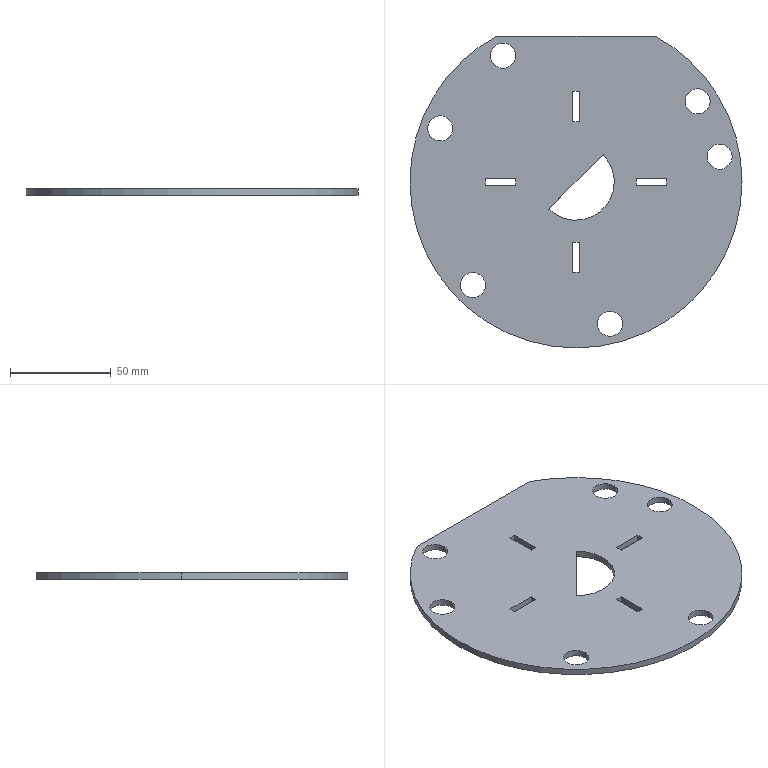Part | SolidWorks | features FlatPattern 1, SMBaseFlange 1, SheetMetal 1 | 1 solid | 36 faces | box 165 x 155 x 3.2 mm | volume 61928 mm3 | plane 20 | cylinder 16 | commonest cylinder face diameters 12.5 x12 165 x3 38.1 x1
STEP:
#1=CARTESIAN_POINT('',(2.418,-3.235,3.2));
#2=VERTEX_POINT('',#1);
#3=CARTESIAN_POINT('',(14.918,-3.235,3.2));
#4=VERTEX_POINT('',#3);
#5=CARTESIAN_POINT('',(8.668,-3.235,3.2));
#6=DIRECTION('',(0.,0.,1.));
#7=DIRECTION('',(1.,0.,0.));
#8=AXIS2_PLACEMENT_3D('',#5,#6,#7);
#9=CIRCLE('',#8,6.25);
#10=EDGE_CURVE('',#2,#4,#9,.T.);
#11=ORIENTED_EDGE('',*,*,#10,.T.);
#12=CARTESIAN_POINT('',(14.918,-3.235,0.));
#13=VERTEX_POINT('',#12);
#14=CARTESIAN_POINT('',(14.918,-3.235,3.2));
#15=DIRECTION('',(0.,0.,-1.));
#16=VECTOR('',#15,1000.);
#17=LINE('',#14,#16);
#18=EDGE_CURVE('',#4,#13,#17,.T.);
#19=ORIENTED_EDGE('',*,*,#18,.T.);
#20=CARTESIAN_POINT('',(2.418,-3.235,0.));
#21=VERTEX_POINT('',#20);
#22=CARTESIAN_POINT('',(8.668,-3.235,0.));
#23=DIRECTION('',(0.,0.,1.));
#24=DIRECTION('',(1.,0.,0.));
#25=AXIS2_PLACEMENT_3D('',#22,#23,#24);
#26=CIRCLE('',#25,6.25);
#27=EDGE_CURVE('',#21,#13,#26,.T.);
#28=ORIENTED_EDGE('',*,*,#27,.F.);
#29=CARTESIAN_POINT('',(2.418,-3.235,3.2));
#30=DIRECTION('',(0.,0.,-1.));
#31=VECTOR('',#30,1000.);
#32=LINE('',#29,#31);
#33=EDGE_CURVE('',#2,#21,#32,.T.);
#34=ORIENTED_EDGE('',*,*,#33,.F.);
#35=EDGE_LOOP('',(#11,#19,#28,#34));
#36=FACE_OUTER_BOUND('',#35,.T.);
#37=CARTESIAN_POINT('',(8.668,-3.235,3.2));
#38=DIRECTION('',(0.,0.,-1.));
#39=DIRECTION('',(-1.,0.,0.));
#40=AXIS2_PLACEMENT_3D('',#37,#38,#39);
#41=CYLINDRICAL_SURFACE('',#40,6.25);
#42=ADVANCED_FACE('',(#36),#41,.F.);
#43=CARTESIAN_POINT('',(-8.524,24.191,3.2));
#44=VERTEX_POINT('',#43);
#45=CARTESIAN_POINT('',(3.976,24.191,3.2));
#46=VERTEX_POINT('',#45);
#47=CARTESIAN_POINT('',(-2.274,24.191,3.2));
#48=DIRECTION('',(0.,0.,1.));
#49=DIRECTION('',(1.,0.,0.));
#50=AXIS2_PLACEMENT_3D('',#47,#48,#49);
#51=CIRCLE('',#50,6.25);
#52=EDGE_CURVE('',#44,#46,#51,.T.);
#53=ORIENTED_EDGE('',*,*,#52,.T.);
#54=CARTESIAN_POINT('',(3.976,24.191,0.));
#55=VERTEX_POINT('',#54);
#56=CARTESIAN_POINT('',(3.976,24.191,3.2));
#57=DIRECTION('',(0.,0.,-1.));
#58=VECTOR('',#57,1000.);
#59=LINE('',#56,#58);
#60=EDGE_CURVE('',#46,#55,#59,.T.);
#61=ORIENTED_EDGE('',*,*,#60,.T.);
#62=CARTESIAN_POINT('',(-8.524,24.191,0.));
#63=VERTEX_POINT('',#62);
#64=CARTESIAN_POINT('',(-2.274,24.191,0.));
#65=DIRECTION('',(0.,0.,1.));
#66=DIRECTION('',(1.,0.,0.));
#67=AXIS2_PLACEMENT_3D('',#64,#65,#66);
#68=CIRCLE('',#67,6.25);
#69=EDGE_CURVE('',#63,#55,#68,.T.);
#70=ORIENTED_EDGE('',*,*,#69,.F.);
#71=CARTESIAN_POINT('',(-8.524,24.191,3.2));
#72=DIRECTION('',(0.,0.,-1.));
#73=VECTOR('',#72,1000.);
#74=LINE('',#71,#73);
#75=EDGE_CURVE('',#44,#63,#74,.T.);
#76=ORIENTED_EDGE('',*,*,#75,.F.);
#77=EDGE_LOOP('',(#53,#61,#70,#76));
#78=FACE_OUTER_BOUND('',#77,.T.);
#79=CARTESIAN_POINT('',(-2.274,24.191,3.2));
#80=DIRECTION('',(0.,0.,-1.));
#81=DIRECTION('',(-1.,0.,0.));
#82=AXIS2_PLACEMENT_3D('',#79,#80,#81);
#83=CYLINDRICAL_SURFACE('',#82,6.25);
#84=ADVANCED_FACE('',(#78),#83,.F.);
#85=CARTESIAN_POINT('',(-105.231,46.962,3.2));
#86=VERTEX_POINT('',#85);
#87=CARTESIAN_POINT('',(-92.731,46.962,3.2));
#88=VERTEX_POINT('',#87);
#89=CARTESIAN_POINT('',(-98.981,46.962,3.2));
#90=DIRECTION('',(0.,0.,1.));
#91=DIRECTION('',(1.,0.,0.));
#92=AXIS2_PLACEMENT_3D('',#89,#90,#91);
#93=CIRCLE('',#92,6.25);
#94=EDGE_CURVE('',#86,#88,#93,.T.);
#95=ORIENTED_EDGE('',*,*,#94,.T.);
#96=CARTESIAN_POINT('',(-92.731,46.962,0.));
#97=VERTEX_POINT('',#96);
#98=CARTESIAN_POINT('',(-92.731,46.962,3.2));
#99=DIRECTION('',(0.,0.,-1.));
#100=VECTOR('',#99,1000.);
#101=LINE('',#98,#100);
#102=EDGE_CURVE('',#88,#97,#101,.T.);
#103=ORIENTED_EDGE('',*,*,#102,.T.);
#104=CARTESIAN_POINT('',(-105.231,46.962,0.));
#105=VERTEX_POINT('',#104);
#106=CARTESIAN_POINT('',(-98.981,46.962,0.));
#107=DIRECTION('',(0.,0.,1.));
#108=DIRECTION('',(1.,0.,0.));
#109=AXIS2_PLACEMENT_3D('',#106,#107,#108);
#110=CIRCLE('',#109,6.25);
#111=EDGE_CURVE('',#105,#97,#110,.T.);
#112=ORIENTED_EDGE('',*,*,#111,.F.);
#113=CARTESIAN_POINT('',(-105.231,46.962,3.2));
#114=DIRECTION('',(0.,0.,-1.));
#115=VECTOR('',#114,1000.);
#116=LINE('',#113,#115);
#117=EDGE_CURVE('',#86,#105,#116,.T.);
#118=ORIENTED_EDGE('',*,*,#117,.F.);
#119=EDGE_LOOP('',(#95,#103,#112,#118));
#120=FACE_OUTER_BOUND('',#119,.T.);
#121=CARTESIAN_POINT('',(-98.981,46.962,3.2));
#122=DIRECTION('',(0.,0.,-1.));
#123=DIRECTION('',(-1.,0.,0.));
#124=AXIS2_PLACEMENT_3D('',#121,#122,#123);
#125=CYLINDRICAL_SURFACE('',#124,6.25);
#126=ADVANCED_FACE('',(#120),#125,.F.);
#127=CARTESIAN_POINT('',(-136.436,10.747,3.2));
#128=VERTEX_POINT('',#127);
#129=CARTESIAN_POINT('',(-123.936,10.747,3.2));
#130=VERTEX_POINT('',#129);
#131=CARTESIAN_POINT('',(-130.186,10.747,3.2));
#132=DIRECTION('',(0.,0.,1.));
#133=DIRECTION('',(1.,0.,0.));
#134=AXIS2_PLACEMENT_3D('',#131,#132,#133);
#135=CIRCLE('',#134,6.25);
#136=EDGE_CURVE('',#128,#130,#135,.T.);
#137=ORIENTED_EDGE('',*,*,#136,.T.);
#138=CARTESIAN_POINT('',(-123.936,10.747,0.));
#139=VERTEX_POINT('',#138);
#140=CARTESIAN_POINT('',(-123.936,10.747,3.2));
#141=DIRECTION('',(0.,0.,-1.));
#142=VECTOR('',#141,1000.);
#143=LINE('',#140,#142);
#144=EDGE_CURVE('',#130,#139,#143,.T.);
#145=ORIENTED_EDGE('',*,*,#144,.T.);
#146=CARTESIAN_POINT('',(-136.436,10.747,0.));
#147=VERTEX_POINT('',#146);
#148=CARTESIAN_POINT('',(-130.186,10.747,0.));
#149=DIRECTION('',(0.,0.,1.));
#150=DIRECTION('',(1.,0.,0.));
#151=AXIS2_PLACEMENT_3D('',#148,#149,#150);
#152=CIRCLE('',#151,6.25);
#153=EDGE_CURVE('',#147,#139,#152,.T.);
#154=ORIENTED_EDGE('',*,*,#153,.F.);
#155=CARTESIAN_POINT('',(-136.436,10.747,3.2));
#156=DIRECTION('',(0.,0.,-1.));
#157=VECTOR('',#156,1000.);
#158=LINE('',#155,#157);
#159=EDGE_CURVE('',#128,#147,#158,.T.);
#160=ORIENTED_EDGE('',*,*,#159,.F.);
#161=EDGE_LOOP('',(#137,#145,#154,#160));
#162=FACE_OUTER_BOUND('',#161,.T.);
#163=CARTESIAN_POINT('',(-130.186,10.747,3.2));
#164=DIRECTION('',(0.,0.,-1.));
#165=DIRECTION('',(-1.,0.,0.));
#166=AXIS2_PLACEMENT_3D('',#163,#164,#165);
#167=CYLINDRICAL_SURFACE('',#166,6.25);
#168=ADVANCED_FACE('',(#162),#167,.F.);
#169=CARTESIAN_POINT('',(-120.246,-67.09,3.2));
#170=VERTEX_POINT('',#169);
#171=CARTESIAN_POINT('',(-107.746,-67.09,3.2));
#172=VERTEX_POINT('',#171);
#173=CARTESIAN_POINT('',(-113.996,-67.09,3.2));
#174=DIRECTION('',(0.,0.,1.));
#175=DIRECTION('',(1.,0.,0.));
#176=AXIS2_PLACEMENT_3D('',#173,#174,#175);
#177=CIRCLE('',#176,6.25);
#178=EDGE_CURVE('',#170,#172,#177,.T.);
#179=ORIENTED_EDGE('',*,*,#178,.T.);
#180=CARTESIAN_POINT('',(-107.746,-67.09,0.));
#181=VERTEX_POINT('',#180);
#182=CARTESIAN_POINT('',(-107.746,-67.09,3.2));
#183=DIRECTION('',(0.,0.,-1.));
#184=VECTOR('',#183,1000.);
#185=LINE('',#182,#184);
#186=EDGE_CURVE('',#172,#181,#185,.T.);
#187=ORIENTED_EDGE('',*,*,#186,.T.);
#188=CARTESIAN_POINT('',(-120.246,-67.09,0.));
#189=VERTEX_POINT('',#188);
#190=CARTESIAN_POINT('',(-113.996,-67.09,0.));
#191=DIRECTION('',(0.,0.,1.));
#192=DIRECTION('',(1.,0.,0.));
#193=AXIS2_PLACEMENT_3D('',#190,#191,#192);
#194=CIRCLE('',#193,6.25);
#195=EDGE_CURVE('',#189,#181,#194,.T.);
#196=ORIENTED_EDGE('',*,*,#195,.F.);
#197=CARTESIAN_POINT('',(-120.246,-67.09,3.2));
#198=DIRECTION('',(0.,0.,-1.));
#199=VECTOR('',#198,1000.);
#200=LINE('',#197,#199);
#201=EDGE_CURVE('',#170,#189,#200,.T.);
#202=ORIENTED_EDGE('',*,*,#201,.F.);
#203=EDGE_LOOP('',(#179,#187,#196,#202));
#204=FACE_OUTER_BOUND('',#203,.T.);
#205=CARTESIAN_POINT('',(-113.996,-67.09,3.2));
#206=DIRECTION('',(0.,0.,-1.));
#207=DIRECTION('',(-1.,0.,0.));
#208=AXIS2_PLACEMENT_3D('',#205,#206,#207);
#209=CYLINDRICAL_SURFACE('',#208,6.25);
#210=ADVANCED_FACE('',(#204),#209,.F.);
#211=CARTESIAN_POINT('',(-52.056,-86.321,3.2));
#212=VERTEX_POINT('',#211);
#213=CARTESIAN_POINT('',(-39.556,-86.321,3.2));
#214=VERTEX_POINT('',#213);
#215=CARTESIAN_POINT('',(-45.806,-86.321,3.2));
#216=DIRECTION('',(0.,0.,1.));
#217=DIRECTION('',(1.,0.,0.));
#218=AXIS2_PLACEMENT_3D('',#215,#216,#217);
#219=CIRCLE('',#218,6.25);
#220=EDGE_CURVE('',#212,#214,#219,.T.);
#221=ORIENTED_EDGE('',*,*,#220,.T.);
#222=CARTESIAN_POINT('',(-39.556,-86.321,0.));
#223=VERTEX_POINT('',#222);
#224=CARTESIAN_POINT('',(-39.556,-86.321,3.2));
#225=DIRECTION('',(0.,0.,-1.));
#226=VECTOR('',#225,1000.);
#227=LINE('',#224,#226);
#228=EDGE_CURVE('',#214,#223,#227,.T.);
#229=ORIENTED_EDGE('',*,*,#228,.T.);
#230=CARTESIAN_POINT('',(-52.056,-86.321,0.));
#231=VERTEX_POINT('',#230);
#232=CARTESIAN_POINT('',(-45.806,-86.321,0.));
#233=DIRECTION('',(0.,0.,1.));
#234=DIRECTION('',(1.,0.,0.));
#235=AXIS2_PLACEMENT_3D('',#232,#233,#234);
#236=CIRCLE('',#235,6.25);
#237=EDGE_CURVE('',#231,#223,#236,.T.);
#238=ORIENTED_EDGE('',*,*,#237,.F.);
#239=CARTESIAN_POINT('',(-52.056,-86.321,3.2));
#240=DIRECTION('',(0.,0.,-1.));
#241=VECTOR('',#240,1000.);
#242=LINE('',#239,#241);
#243=EDGE_CURVE('',#212,#231,#242,.T.);
#244=ORIENTED_EDGE('',*,*,#243,.F.);
#245=EDGE_LOOP('',(#221,#229,#238,#244));
#246=FACE_OUTER_BOUND('',#245,.T.);
#247=CARTESIAN_POINT('',(-45.806,-86.321,3.2));
#248=DIRECTION('',(0.,0.,-1.));
#249=DIRECTION('',(-1.,0.,0.));
#250=AXIS2_PLACEMENT_3D('',#247,#248,#249);
#251=CYLINDRICAL_SURFACE('',#250,6.25);
#252=ADVANCED_FACE('',(#246),#251,.F.);
#253=CARTESIAN_POINT('',(19.769,-15.825,3.2));
#254=VERTEX_POINT('',#253);
#255=CARTESIAN_POINT('',(-23.361,56.675,3.2));
#256=VERTEX_POINT('',#255);
#257=CARTESIAN_POINT('',(-62.731,-15.825,3.2));
#258=DIRECTION('',(0.,0.,1.));
#259=DIRECTION('',(1.,0.,0.));
#260=AXIS2_PLACEMENT_3D('',#257,#258,#259);
#261=CIRCLE('',#260,82.5);
#262=EDGE_CURVE('',#254,#256,#261,.T.);
#263=ORIENTED_EDGE('',*,*,#262,.F.);
#264=CARTESIAN_POINT('',(19.769,-15.825,0.));
#265=VERTEX_POINT('',#264);
#266=CARTESIAN_POINT('',(19.769,-15.825,3.2));
#267=DIRECTION('',(0.,0.,-1.));
#268=VECTOR('',#267,1000.);
#269=LINE('',#266,#268);
#270=EDGE_CURVE('',#254,#265,#269,.T.);
#271=ORIENTED_EDGE('',*,*,#270,.T.);
#272=CARTESIAN_POINT('',(-23.361,56.675,0.));
#273=VERTEX_POINT('',#272);
#274=CARTESIAN_POINT('',(-62.731,-15.825,0.));
#275=DIRECTION('',(0.,0.,1.));
#276=DIRECTION('',(1.,0.,0.));
#277=AXIS2_PLACEMENT_3D('',#274,#275,#276);
#278=CIRCLE('',#277,82.5);
#279=EDGE_CURVE('',#265,#273,#278,.T.);
#280=ORIENTED_EDGE('',*,*,#279,.T.);
#281=CARTESIAN_POINT('',(-23.361,56.675,3.2));
#282=DIRECTION('',(0.,0.,-1.));
#283=VECTOR('',#282,1000.);
#284=LINE('',#281,#283);
#285=EDGE_CURVE('',#256,#273,#284,.T.);
#286=ORIENTED_EDGE('',*,*,#285,.F.);
#287=EDGE_LOOP('',(#263,#271,#280,#286));
#288=FACE_OUTER_BOUND('',#287,.T.);
#289=CARTESIAN_POINT('',(-62.731,-15.825,3.2));
#290=DIRECTION('',(0.,0.,-1.));
#291=DIRECTION('',(-1.,0.,0.));
#292=AXIS2_PLACEMENT_3D('',#289,#290,#291);
#293=CYLINDRICAL_SURFACE('',#292,82.5);
#294=ADVANCED_FACE('',(#288),#293,.T.);
#295=ORIENTED_EDGE('',*,*,#270,.F.);
#296=CARTESIAN_POINT('',(-145.231,-15.825,3.2));
#297=VERTEX_POINT('',#296);
#298=CARTESIAN_POINT('',(-62.731,-15.825,3.2));
#299=DIRECTION('',(0.,0.,1.));
#300=DIRECTION('',(1.,0.,0.));
#301=AXIS2_PLACEMENT_3D('',#298,#299,#300);
#302=CIRCLE('',#301,82.5);
#303=EDGE_CURVE('',#297,#254,#302,.T.);
#304=ORIENTED_EDGE('',*,*,#303,.F.);
#305=CARTESIAN_POINT('',(-145.231,-15.825,0.));
#306=VERTEX_POINT('',#305);
#307=CARTESIAN_POINT('',(-145.231,-15.825,3.2));
#308=DIRECTION('',(0.,0.,-1.));
#309=VECTOR('',#308,1000.);
#310=LINE('',#307,#309);
#311=EDGE_CURVE('',#297,#306,#310,.T.);
#312=ORIENTED_EDGE('',*,*,#311,.T.);
#313=CARTESIAN_POINT('',(-62.731,-15.825,0.));
#314=DIRECTION('',(0.,0.,1.));
#315=DIRECTION('',(1.,0.,0.));
#316=AXIS2_PLACEMENT_3D('',#313,#314,#315);
#317=CIRCLE('',#316,82.5);
#318=EDGE_CURVE('',#306,#265,#317,.T.);
#319=ORIENTED_EDGE('',*,*,#318,.T.);
#320=EDGE_LOOP('',(#295,#304,#312,#319));
#321=FACE_OUTER_BOUND('',#320,.T.);
#322=CARTESIAN_POINT('',(-62.731,-15.825,3.2));
#323=DIRECTION('',(0.,0.,-1.));
#324=DIRECTION('',(-1.,0.,0.));
#325=AXIS2_PLACEMENT_3D('',#322,#323,#324);
#326=CYLINDRICAL_SURFACE('',#325,82.5);
#327=ADVANCED_FACE('',(#321),#326,.T.);
#328=ORIENTED_EDGE('',*,*,#52,.F.);
#329=CARTESIAN_POINT('',(-2.274,24.191,3.2));
#330=DIRECTION('',(0.,0.,1.));
#331=DIRECTION('',(1.,0.,0.));
#332=AXIS2_PLACEMENT_3D('',#329,#330,#331);
#333=CIRCLE('',#332,6.25);
#334=EDGE_CURVE('',#46,#44,#333,.T.);
#335=ORIENTED_EDGE('',*,*,#334,.F.);
#336=EDGE_LOOP('',(#328,#335));
#337=FACE_BOUND('',#336,.T.);
#338=ORIENTED_EDGE('',*,*,#136,.F.);
#339=CARTESIAN_POINT('',(-130.186,10.747,3.2));
#340=DIRECTION('',(0.,0.,1.));
#341=DIRECTION('',(1.,0.,0.));
#342=AXIS2_PLACEMENT_3D('',#339,#340,#341);
#343=CIRCLE('',#342,6.25);
#344=EDGE_CURVE('',#130,#128,#343,.T.);
#345=ORIENTED_EDGE('',*,*,#344,.F.);
#346=EDGE_LOOP('',(#338,#345));
#347=FACE_BOUND('',#346,.T.);
#348=ORIENTED_EDGE('',*,*,#220,.F.);
#349=CARTESIAN_POINT('',(-45.806,-86.321,3.2));
#350=DIRECTION('',(0.,0.,1.));
#351=DIRECTION('',(1.,0.,0.));
#352=AXIS2_PLACEMENT_3D('',#349,#350,#351);
#353=CIRCLE('',#352,6.25);
#354=EDGE_CURVE('',#214,#212,#353,.T.);
#355=ORIENTED_EDGE('',*,*,#354,.F.);
#356=EDGE_LOOP('',(#348,#355));
#357=FACE_BOUND('',#356,.T.);
#358=CARTESIAN_POINT('',(-102.101,56.675,3.2));
#359=VERTEX_POINT('',#358);
#360=CARTESIAN_POINT('',(-62.731,-15.825,3.2));
#361=DIRECTION('',(0.,0.,1.));
#362=DIRECTION('',(1.,0.,0.));
#363=AXIS2_PLACEMENT_3D('',#360,#361,#362);
#364=CIRCLE('',#363,82.5);
#365=EDGE_CURVE('',#359,#297,#364,.T.);
#366=ORIENTED_EDGE('',*,*,#365,.T.);
#367=ORIENTED_EDGE('',*,*,#303,.T.);
#368=ORIENTED_EDGE('',*,*,#262,.T.);
#369=CARTESIAN_POINT('',(-23.361,56.675,3.2));
#370=DIRECTION('',(-1.,0.,0.));
#371=VECTOR('',#370,1000.);
#372=LINE('',#369,#371);
#373=EDGE_CURVE('',#256,#359,#372,.T.);
#374=ORIENTED_EDGE('',*,*,#373,.T.);
#375=EDGE_LOOP('',(#366,#367,#368,#374));
#376=FACE_OUTER_BOUND('',#375,.T.);
#377=CARTESIAN_POINT('',(-32.731,-17.425,3.2));
#378=VERTEX_POINT('',#377);
#379=CARTESIAN_POINT('',(-17.731,-17.425,3.2));
#380=VERTEX_POINT('',#379);
#381=CARTESIAN_POINT('',(-32.731,-17.425,3.2));
#382=DIRECTION('',(1.,0.,0.));
#383=VECTOR('',#382,1000.);
#384=LINE('',#381,#383);
#385=EDGE_CURVE('',#378,#380,#384,.T.);
#386=ORIENTED_EDGE('',*,*,#385,.F.);
#387=CARTESIAN_POINT('',(-32.731,-14.225,3.2));
#388=VERTEX_POINT('',#387);
#389=CARTESIAN_POINT('',(-32.731,-14.225,3.2));
#390=DIRECTION('',(0.,-1.,0.));
#391=VECTOR('',#390,1000.);
#392=LINE('',#389,#391);
#393=EDGE_CURVE('',#388,#378,#392,.T.);
#394=ORIENTED_EDGE('',*,*,#393,.F.);
#395=CARTESIAN_POINT('',(-17.731,-14.225,3.2));
#396=VERTEX_POINT('',#395);
#397=CARTESIAN_POINT('',(-32.731,-14.225,3.2));
#398=DIRECTION('',(-1.,0.,0.));
#399=VECTOR('',#398,1000.);
#400=LINE('',#397,#399);
#401=EDGE_CURVE('',#396,#388,#400,.T.);
#402=ORIENTED_EDGE('',*,*,#401,.F.);
#403=CARTESIAN_POINT('',(-17.731,-14.225,3.2));
#404=DIRECTION('',(0.,1.,0.));
#405=VECTOR('',#404,1000.);
#406=LINE('',#403,#405);
#407=EDGE_CURVE('',#380,#396,#406,.T.);
#408=ORIENTED_EDGE('',*,*,#407,.F.);
#409=EDGE_LOOP('',(#386,#394,#402,#408));
#410=FACE_BOUND('',#409,.T.);
#411=CARTESIAN_POINT('',(-49.261,-2.354,3.2));
#412=VERTEX_POINT('',#411);
#413=CARTESIAN_POINT('',(-76.201,-29.295,3.2));
#414=VERTEX_POINT('',#413);
#415=CARTESIAN_POINT('',(-49.261,-2.354,3.2));
#416=DIRECTION('',(-0.7071,-0.7071,0.));
#417=VECTOR('',#416,1000.);
#418=LINE('',#415,#417);
#419=EDGE_CURVE('',#412,#414,#418,.T.);
#420=ORIENTED_EDGE('',*,*,#419,.F.);
#421=CARTESIAN_POINT('',(-62.731,-15.825,3.2));
#422=DIRECTION('',(0.,0.,1.));
#423=DIRECTION('',(1.,0.,0.));
#424=AXIS2_PLACEMENT_3D('',#421,#422,#423);
#425=CIRCLE('',#424,19.05);
#426=EDGE_CURVE('',#414,#412,#425,.T.);
#427=ORIENTED_EDGE('',*,*,#426,.F.);
#428=EDGE_LOOP('',(#420,#427));
#429=FACE_BOUND('',#428,.T.);
#430=ORIENTED_EDGE('',*,*,#178,.F.);
#431=CARTESIAN_POINT('',(-113.996,-67.09,3.2));
#432=DIRECTION('',(0.,0.,1.));
#433=DIRECTION('',(1.,0.,0.));
#434=AXIS2_PLACEMENT_3D('',#431,#432,#433);
#435=CIRCLE('',#434,6.25);
#436=EDGE_CURVE('',#172,#170,#435,.T.);
#437=ORIENTED_EDGE('',*,*,#436,.F.);
#438=EDGE_LOOP('',(#430,#437));
#439=FACE_BOUND('',#438,.T.);
#440=ORIENTED_EDGE('',*,*,#94,.F.);
#441=CARTESIAN_POINT('',(-98.981,46.962,3.2));
#442=DIRECTION('',(0.,0.,1.));
#443=DIRECTION('',(1.,0.,0.));
#444=AXIS2_PLACEMENT_3D('',#441,#442,#443);
#445=CIRCLE('',#444,6.25);
#446=EDGE_CURVE('',#88,#86,#445,.T.);
#447=ORIENTED_EDGE('',*,*,#446,.F.);
#448=EDGE_LOOP('',(#440,#447));
#449=FACE_BOUND('',#448,.T.);
#450=ORIENTED_EDGE('',*,*,#10,.F.);
#451=CARTESIAN_POINT('',(8.668,-3.235,3.2));
#452=DIRECTION('',(0.,0.,1.));
#453=DIRECTION('',(1.,0.,0.));
#454=AXIS2_PLACEMENT_3D('',#451,#452,#453);
#455=CIRCLE('',#454,6.25);
#456=EDGE_CURVE('',#4,#2,#455,.T.);
#457=ORIENTED_EDGE('',*,*,#456,.F.);
#458=EDGE_LOOP('',(#450,#457));
#459=FACE_BOUND('',#458,.T.);
#460=CARTESIAN_POINT('',(-64.331,-60.825,3.2));
#461=VERTEX_POINT('',#460);
#462=CARTESIAN_POINT('',(-61.131,-60.825,3.2));
#463=VERTEX_POINT('',#462);
#464=CARTESIAN_POINT('',(-64.331,-60.825,3.2));
#465=DIRECTION('',(1.,0.,0.));
#466=VECTOR('',#465,1000.);
#467=LINE('',#464,#466);
#468=EDGE_CURVE('',#461,#463,#467,.T.);
#469=ORIENTED_EDGE('',*,*,#468,.F.);
#470=CARTESIAN_POINT('',(-64.331,-45.825,3.2));
#471=VERTEX_POINT('',#470);
#472=CARTESIAN_POINT('',(-64.331,-45.825,3.2));
#473=DIRECTION('',(0.,-1.,0.));
#474=VECTOR('',#473,1000.);
#475=LINE('',#472,#474);
#476=EDGE_CURVE('',#471,#461,#475,.T.);
#477=ORIENTED_EDGE('',*,*,#476,.F.);
#478=CARTESIAN_POINT('',(-61.131,-45.825,3.2));
#479=VERTEX_POINT('',#478);
#480=CARTESIAN_POINT('',(-64.331,-45.825,3.2));
#481=DIRECTION('',(-1.,0.,0.));
#482=VECTOR('',#481,1000.);
#483=LINE('',#480,#482);
#484=EDGE_CURVE('',#479,#471,#483,.T.);
#485=ORIENTED_EDGE('',*,*,#484,.F.);
#486=CARTESIAN_POINT('',(-61.131,-45.825,3.2));
#487=DIRECTION('',(0.,1.,0.));
#488=VECTOR('',#487,1000.);
#489=LINE('',#486,#488);
#490=EDGE_CURVE('',#463,#479,#489,.T.);
#491=ORIENTED_EDGE('',*,*,#490,.F.);
#492=EDGE_LOOP('',(#469,#477,#485,#491));
#493=FACE_BOUND('',#492,.T.);
#494=CARTESIAN_POINT('',(-92.731,-14.225,3.2));
#495=VERTEX_POINT('',#494);
#496=CARTESIAN_POINT('',(-107.731,-14.225,3.2));
#497=VERTEX_POINT('',#496);
#498=CARTESIAN_POINT('',(-92.731,-14.225,3.2));
#499=DIRECTION('',(-1.,0.,0.));
#500=VECTOR('',#499,1000.);
#501=LINE('',#498,#500);
#502=EDGE_CURVE('',#495,#497,#501,.T.);
#503=ORIENTED_EDGE('',*,*,#502,.F.);
#504=CARTESIAN_POINT('',(-92.731,-17.425,3.2));
#505=VERTEX_POINT('',#504);
#506=CARTESIAN_POINT('',(-92.731,-14.225,3.2));
#507=DIRECTION('',(0.,1.,0.));
#508=VECTOR('',#507,1000.);
#509=LINE('',#506,#508);
#510=EDGE_CURVE('',#505,#495,#509,.T.);
#511=ORIENTED_EDGE('',*,*,#510,.F.);
#512=CARTESIAN_POINT('',(-107.731,-17.425,3.2));
#513=VERTEX_POINT('',#512);
#514=CARTESIAN_POINT('',(-92.731,-17.425,3.2));
#515=DIRECTION('',(1.,0.,0.));
#516=VECTOR('',#515,1000.);
#517=LINE('',#514,#516);
#518=EDGE_CURVE('',#513,#505,#517,.T.);
#519=ORIENTED_EDGE('',*,*,#518,.F.);
#520=CARTESIAN_POINT('',(-107.731,-14.225,3.2));
#521=DIRECTION('',(0.,-1.,0.));
#522=VECTOR('',#521,1000.);
#523=LINE('',#520,#522);
#524=EDGE_CURVE('',#497,#513,#523,.T.);
#525=ORIENTED_EDGE('',*,*,#524,.F.);
#526=EDGE_LOOP('',(#503,#511,#519,#525));
#527=FACE_BOUND('',#526,.T.);
#528=CARTESIAN_POINT('',(-64.331,14.175,3.2));
#529=VERTEX_POINT('',#528);
#530=CARTESIAN_POINT('',(-61.131,14.175,3.2));
#531=VERTEX_POINT('',#530);
#532=CARTESIAN_POINT('',(-64.331,14.175,3.2));
#533=DIRECTION('',(1.,0.,0.));
#534=VECTOR('',#533,1000.);
#535=LINE('',#532,#534);
#536=EDGE_CURVE('',#529,#531,#535,.T.);
#537=ORIENTED_EDGE('',*,*,#536,.F.);
#538=CARTESIAN_POINT('',(-64.331,29.175,3.2));
#539=VERTEX_POINT('',#538);
#540=CARTESIAN_POINT('',(-64.331,14.175,3.2));
#541=DIRECTION('',(0.,-1.,0.));
#542=VECTOR('',#541,1000.);
#543=LINE('',#540,#542);
#544=EDGE_CURVE('',#539,#529,#543,.T.);
#545=ORIENTED_EDGE('',*,*,#544,.F.);
#546=CARTESIAN_POINT('',(-61.131,29.175,3.2));
#547=VERTEX_POINT('',#546);
#548=CARTESIAN_POINT('',(-64.331,29.175,3.2));
#549=DIRECTION('',(-1.,0.,0.));
#550=VECTOR('',#549,1000.);
#551=LINE('',#548,#550);
#552=EDGE_CURVE('',#547,#539,#551,.T.);
#553=ORIENTED_EDGE('',*,*,#552,.F.);
#554=CARTESIAN_POINT('',(-61.131,14.175,3.2));
#555=DIRECTION('',(0.,1.,0.));
#556=VECTOR('',#555,1000.);
#557=LINE('',#554,#556);
#558=EDGE_CURVE('',#531,#547,#557,.T.);
#559=ORIENTED_EDGE('',*,*,#558,.F.);
#560=EDGE_LOOP('',(#537,#545,#553,#559));
#561=FACE_BOUND('',#560,.T.);
#562=CARTESIAN_POINT('',(-62.731,-15.825,3.2));
#563=DIRECTION('',(0.,0.,1.));
#564=DIRECTION('',(1.,0.,0.));
#565=AXIS2_PLACEMENT_3D('',#562,#563,#564);
#566=PLANE('',#565);
#567=ADVANCED_FACE('',(#337,#347,#357,#376,#410,#429,#439,#449,#459,#493,#527,#561),#566,.T.);
#568=CARTESIAN_POINT('',(-92.731,-17.425,0.));
#569=VERTEX_POINT('',#568);
#570=CARTESIAN_POINT('',(-92.731,-14.225,0.));
#571=VERTEX_POINT('',#570);
#572=CARTESIAN_POINT('',(-92.731,-14.225,0.));
#573=DIRECTION('',(0.,1.,0.));
#574=VECTOR('',#573,1000.);
#575=LINE('',#572,#574);
#576=EDGE_CURVE('',#569,#571,#575,.T.);
#577=ORIENTED_EDGE('',*,*,#576,.T.);
#578=CARTESIAN_POINT('',(-107.731,-14.225,0.));
#579=VERTEX_POINT('',#578);
#580=CARTESIAN_POINT('',(-92.731,-14.225,0.));
#581=DIRECTION('',(-1.,0.,0.));
#582=VECTOR('',#581,1000.);
#583=LINE('',#580,#582);
#584=EDGE_CURVE('',#571,#579,#583,.T.);
#585=ORIENTED_EDGE('',*,*,#584,.T.);
#586=CARTESIAN_POINT('',(-107.731,-17.425,0.));
#587=VERTEX_POINT('',#586);
#588=CARTESIAN_POINT('',(-107.731,-14.225,0.));
#589=DIRECTION('',(0.,-1.,0.));
#590=VECTOR('',#589,1000.);
#591=LINE('',#588,#590);
#592=EDGE_CURVE('',#579,#587,#591,.T.);
#593=ORIENTED_EDGE('',*,*,#592,.T.);
#594=CARTESIAN_POINT('',(-92.731,-17.425,0.));
#595=DIRECTION('',(1.,0.,0.));
#596=VECTOR('',#595,1000.);
#597=LINE('',#594,#596);
#598=EDGE_CURVE('',#587,#569,#597,.T.);
#599=ORIENTED_EDGE('',*,*,#598,.T.);
#600=EDGE_LOOP('',(#577,#585,#593,#599));
#601=FACE_BOUND('',#600,.T.);
#602=ORIENTED_EDGE('',*,*,#27,.T.);
#603=CARTESIAN_POINT('',(8.668,-3.235,0.));
#604=DIRECTION('',(0.,0.,1.));
#605=DIRECTION('',(1.,0.,0.));
#606=AXIS2_PLACEMENT_3D('',#603,#604,#605);
#607=CIRCLE('',#606,6.25);
#608=EDGE_CURVE('',#13,#21,#607,.T.);
#609=ORIENTED_EDGE('',*,*,#608,.T.);
#610=EDGE_LOOP('',(#602,#609));
#611=FACE_BOUND('',#610,.T.);
#612=ORIENTED_EDGE('',*,*,#69,.T.);
#613=CARTESIAN_POINT('',(-2.274,24.191,0.));
#614=DIRECTION('',(0.,0.,1.));
#615=DIRECTION('',(1.,0.,0.));
#616=AXIS2_PLACEMENT_3D('',#613,#614,#615);
#617=CIRCLE('',#616,6.25);
#618=EDGE_CURVE('',#55,#63,#617,.T.);
#619=ORIENTED_EDGE('',*,*,#618,.T.);
#620=EDGE_LOOP('',(#612,#619));
#621=FACE_BOUND('',#620,.T.);
#622=ORIENTED_EDGE('',*,*,#111,.T.);
#623=CARTESIAN_POINT('',(-98.981,46.962,0.));
#624=DIRECTION('',(0.,0.,1.));
#625=DIRECTION('',(1.,0.,0.));
#626=AXIS2_PLACEMENT_3D('',#623,#624,#625);
#627=CIRCLE('',#626,6.25);
#628=EDGE_CURVE('',#97,#105,#627,.T.);
#629=ORIENTED_EDGE('',*,*,#628,.T.);
#630=EDGE_LOOP('',(#622,#629));
#631=FACE_BOUND('',#630,.T.);
#632=ORIENTED_EDGE('',*,*,#153,.T.);
#633=CARTESIAN_POINT('',(-130.186,10.747,0.));
#634=DIRECTION('',(0.,0.,1.));
#635=DIRECTION('',(1.,0.,0.));
#636=AXIS2_PLACEMENT_3D('',#633,#634,#635);
#637=CIRCLE('',#636,6.25);
#638=EDGE_CURVE('',#139,#147,#637,.T.);
#639=ORIENTED_EDGE('',*,*,#638,.T.);
#640=EDGE_LOOP('',(#632,#639));
#641=FACE_BOUND('',#640,.T.);
#642=ORIENTED_EDGE('',*,*,#195,.T.);
#643=CARTESIAN_POINT('',(-113.996,-67.09,0.));
#644=DIRECTION('',(0.,0.,1.));
#645=DIRECTION('',(1.,0.,0.));
#646=AXIS2_PLACEMENT_3D('',#643,#644,#645);
#647=CIRCLE('',#646,6.25);
#648=EDGE_CURVE('',#181,#189,#647,.T.);
#649=ORIENTED_EDGE('',*,*,#648,.T.);
#650=EDGE_LOOP('',(#642,#649));
#651=FACE_BOUND('',#650,.T.);
#652=ORIENTED_EDGE('',*,*,#237,.T.);
#653=CARTESIAN_POINT('',(-45.806,-86.321,0.));
#654=DIRECTION('',(0.,0.,1.));
#655=DIRECTION('',(1.,0.,0.));
#656=AXIS2_PLACEMENT_3D('',#653,#654,#655);
#657=CIRCLE('',#656,6.25);
#658=EDGE_CURVE('',#223,#231,#657,.T.);
#659=ORIENTED_EDGE('',*,*,#658,.T.);
#660=EDGE_LOOP('',(#652,#659));
#661=FACE_BOUND('',#660,.T.);
#662=CARTESIAN_POINT('',(-76.201,-29.295,0.));
#663=VERTEX_POINT('',#662);
#664=CARTESIAN_POINT('',(-49.261,-2.354,0.));
#665=VERTEX_POINT('',#664);
#666=CARTESIAN_POINT('',(-62.731,-15.825,0.));
#667=DIRECTION('',(0.,0.,1.));
#668=DIRECTION('',(1.,0.,0.));
#669=AXIS2_PLACEMENT_3D('',#666,#667,#668);
#670=CIRCLE('',#669,19.05);
#671=EDGE_CURVE('',#663,#665,#670,.T.);
#672=ORIENTED_EDGE('',*,*,#671,.T.);
#673=CARTESIAN_POINT('',(-49.261,-2.354,0.));
#674=DIRECTION('',(-0.7071,-0.7071,0.));
#675=VECTOR('',#674,1000.);
#676=LINE('',#673,#675);
#677=EDGE_CURVE('',#665,#663,#676,.T.);
#678=ORIENTED_EDGE('',*,*,#677,.T.);
#679=EDGE_LOOP('',(#672,#678));
#680=FACE_BOUND('',#679,.T.);
#681=CARTESIAN_POINT('',(-102.101,56.675,0.));
#682=VERTEX_POINT('',#681);
#683=CARTESIAN_POINT('',(-62.731,-15.825,0.));
#684=DIRECTION('',(0.,0.,1.));
#685=DIRECTION('',(1.,0.,0.));
#686=AXIS2_PLACEMENT_3D('',#683,#684,#685);
#687=CIRCLE('',#686,82.5);
#688=EDGE_CURVE('',#682,#306,#687,.T.);
#689=ORIENTED_EDGE('',*,*,#688,.F.);
#690=CARTESIAN_POINT('',(-23.361,56.675,0.));
#691=DIRECTION('',(-1.,0.,0.));
#692=VECTOR('',#691,1000.);
#693=LINE('',#690,#692);
#694=EDGE_CURVE('',#273,#682,#693,.T.);
#695=ORIENTED_EDGE('',*,*,#694,.F.);
#696=ORIENTED_EDGE('',*,*,#279,.F.);
#697=ORIENTED_EDGE('',*,*,#318,.F.);
#698=EDGE_LOOP('',(#689,#695,#696,#697));
#699=FACE_OUTER_BOUND('',#698,.T.);
#700=CARTESIAN_POINT('',(-32.731,-14.225,0.));
#701=VERTEX_POINT('',#700);
#702=CARTESIAN_POINT('',(-32.731,-17.425,0.));
#703=VERTEX_POINT('',#702);
#704=CARTESIAN_POINT('',(-32.731,-14.225,0.));
#705=DIRECTION('',(0.,-1.,0.));
#706=VECTOR('',#705,1000.);
#707=LINE('',#704,#706);
#708=EDGE_CURVE('',#701,#703,#707,.T.);
#709=ORIENTED_EDGE('',*,*,#708,.T.);
#710=CARTESIAN_POINT('',(-17.731,-17.425,0.));
#711=VERTEX_POINT('',#710);
#712=CARTESIAN_POINT('',(-32.731,-17.425,0.));
#713=DIRECTION('',(1.,0.,0.));
#714=VECTOR('',#713,1000.);
#715=LINE('',#712,#714);
#716=EDGE_CURVE('',#703,#711,#715,.T.);
#717=ORIENTED_EDGE('',*,*,#716,.T.);
#718=CARTESIAN_POINT('',(-17.731,-14.225,0.));
#719=VERTEX_POINT('',#718);
#720=CARTESIAN_POINT('',(-17.731,-14.225,0.));
#721=DIRECTION('',(0.,1.,0.));
#722=VECTOR('',#721,1000.);
#723=LINE('',#720,#722);
#724=EDGE_CURVE('',#711,#719,#723,.T.);
#725=ORIENTED_EDGE('',*,*,#724,.T.);
#726=CARTESIAN_POINT('',(-32.731,-14.225,0.));
#727=DIRECTION('',(-1.,0.,0.));
#728=VECTOR('',#727,1000.);
#729=LINE('',#726,#728);
#730=EDGE_CURVE('',#719,#701,#729,.T.);
#731=ORIENTED_EDGE('',*,*,#730,.T.);
#732=EDGE_LOOP('',(#709,#717,#725,#731));
#733=FACE_BOUND('',#732,.T.);
#734=CARTESIAN_POINT('',(-64.331,-45.825,0.));
#735=VERTEX_POINT('',#734);
#736=CARTESIAN_POINT('',(-64.331,-60.825,0.));
#737=VERTEX_POINT('',#736);
#738=CARTESIAN_POINT('',(-64.331,-45.825,0.));
#739=DIRECTION('',(0.,-1.,0.));
#740=VECTOR('',#739,1000.);
#741=LINE('',#738,#740);
#742=EDGE_CURVE('',#735,#737,#741,.T.);
#743=ORIENTED_EDGE('',*,*,#742,.T.);
#744=CARTESIAN_POINT('',(-61.131,-60.825,0.));
#745=VERTEX_POINT('',#744);
#746=CARTESIAN_POINT('',(-64.331,-60.825,0.));
#747=DIRECTION('',(1.,0.,0.));
#748=VECTOR('',#747,1000.);
#749=LINE('',#746,#748);
#750=EDGE_CURVE('',#737,#745,#749,.T.);
#751=ORIENTED_EDGE('',*,*,#750,.T.);
#752=CARTESIAN_POINT('',(-61.131,-45.825,0.));
#753=VERTEX_POINT('',#752);
#754=CARTESIAN_POINT('',(-61.131,-45.825,0.));
#755=DIRECTION('',(0.,1.,0.));
#756=VECTOR('',#755,1000.);
#757=LINE('',#754,#756);
#758=EDGE_CURVE('',#745,#753,#757,.T.);
#759=ORIENTED_EDGE('',*,*,#758,.T.);
#760=CARTESIAN_POINT('',(-64.331,-45.825,0.));
#761=DIRECTION('',(-1.,0.,0.));
#762=VECTOR('',#761,1000.);
#763=LINE('',#760,#762);
#764=EDGE_CURVE('',#753,#735,#763,.T.);
#765=ORIENTED_EDGE('',*,*,#764,.T.);
#766=EDGE_LOOP('',(#743,#751,#759,#765));
#767=FACE_BOUND('',#766,.T.);
#768=CARTESIAN_POINT('',(-64.331,29.175,0.));
#769=VERTEX_POINT('',#768);
#770=CARTESIAN_POINT('',(-64.331,14.175,0.));
#771=VERTEX_POINT('',#770);
#772=CARTESIAN_POINT('',(-64.331,14.175,0.));
#773=DIRECTION('',(0.,-1.,0.));
#774=VECTOR('',#773,1000.);
#775=LINE('',#772,#774);
#776=EDGE_CURVE('',#769,#771,#775,.T.);
#777=ORIENTED_EDGE('',*,*,#776,.T.);
#778=CARTESIAN_POINT('',(-61.131,14.175,0.));
#779=VERTEX_POINT('',#778);
#780=CARTESIAN_POINT('',(-64.331,14.175,0.));
#781=DIRECTION('',(1.,0.,0.));
#782=VECTOR('',#781,1000.);
#783=LINE('',#780,#782);
#784=EDGE_CURVE('',#771,#779,#783,.T.);
#785=ORIENTED_EDGE('',*,*,#784,.T.);
#786=CARTESIAN_POINT('',(-61.131,29.175,0.));
#787=VERTEX_POINT('',#786);
#788=CARTESIAN_POINT('',(-61.131,14.175,0.));
#789=DIRECTION('',(0.,1.,0.));
#790=VECTOR('',#789,1000.);
#791=LINE('',#788,#790);
#792=EDGE_CURVE('',#779,#787,#791,.T.);
#793=ORIENTED_EDGE('',*,*,#792,.T.);
#794=CARTESIAN_POINT('',(-64.331,29.175,0.));
#795=DIRECTION('',(-1.,0.,0.));
#796=VECTOR('',#795,1000.);
#797=LINE('',#794,#796);
#798=EDGE_CURVE('',#787,#769,#797,.T.);
#799=ORIENTED_EDGE('',*,*,#798,.T.);
#800=EDGE_LOOP('',(#777,#785,#793,#799));
#801=FACE_BOUND('',#800,.T.);
#802=CARTESIAN_POINT('',(-62.731,-15.825,0.));
#803=DIRECTION('',(0.,0.,1.));
#804=DIRECTION('',(1.,0.,0.));
#805=AXIS2_PLACEMENT_3D('',#802,#803,#804);
#806=PLANE('',#805);
#807=ADVANCED_FACE('',(#601,#611,#621,#631,#641,#651,#661,#680,#699,#733,#767,#801),#806,.F.);
#808=ORIENTED_EDGE('',*,*,#311,.F.);
#809=ORIENTED_EDGE('',*,*,#365,.F.);
#810=CARTESIAN_POINT('',(-102.101,56.675,3.2));
#811=DIRECTION('',(0.,0.,-1.));
#812=VECTOR('',#811,1000.);
#813=LINE('',#810,#812);
#814=EDGE_CURVE('',#359,#682,#813,.T.);
#815=ORIENTED_EDGE('',*,*,#814,.T.);
#816=ORIENTED_EDGE('',*,*,#688,.T.);
#817=EDGE_LOOP('',(#808,#809,#815,#816));
#818=FACE_OUTER_BOUND('',#817,.T.);
#819=CARTESIAN_POINT('',(-62.731,-15.825,3.2));
#820=DIRECTION('',(0.,0.,-1.));
#821=DIRECTION('',(-1.,0.,0.));
#822=AXIS2_PLACEMENT_3D('',#819,#820,#821);
#823=CYLINDRICAL_SURFACE('',#822,82.5);
#824=ADVANCED_FACE('',(#818),#823,.T.);
#825=ORIENTED_EDGE('',*,*,#694,.T.);
#826=ORIENTED_EDGE('',*,*,#814,.F.);
#827=ORIENTED_EDGE('',*,*,#373,.F.);
#828=ORIENTED_EDGE('',*,*,#285,.T.);
#829=EDGE_LOOP('',(#825,#826,#827,#828));
#830=FACE_OUTER_BOUND('',#829,.T.);
#831=CARTESIAN_POINT('',(-23.361,56.675,3.2));
#832=DIRECTION('',(0.,-1.,0.));
#833=DIRECTION('',(0.,0.,-1.));
#834=AXIS2_PLACEMENT_3D('',#831,#832,#833);
#835=PLANE('',#834);
#836=ADVANCED_FACE('',(#830),#835,.F.);
#837=ORIENTED_EDGE('',*,*,#708,.F.);
#838=CARTESIAN_POINT('',(-32.731,-14.225,3.2));
#839=DIRECTION('',(0.,0.,-1.));
#840=VECTOR('',#839,1000.);
#841=LINE('',#838,#840);
#842=EDGE_CURVE('',#388,#701,#841,.T.);
#843=ORIENTED_EDGE('',*,*,#842,.F.);
#844=ORIENTED_EDGE('',*,*,#393,.T.);
#845=CARTESIAN_POINT('',(-32.731,-17.425,3.2));
#846=DIRECTION('',(0.,0.,-1.));
#847=VECTOR('',#846,1000.);
#848=LINE('',#845,#847);
#849=EDGE_CURVE('',#378,#703,#848,.T.);
#850=ORIENTED_EDGE('',*,*,#849,.T.);
#851=EDGE_LOOP('',(#837,#843,#844,#850));
#852=FACE_OUTER_BOUND('',#851,.T.);
#853=CARTESIAN_POINT('',(-32.731,-14.225,3.2));
#854=DIRECTION('',(1.,0.,0.));
#855=DIRECTION('',(0.,0.,-1.));
#856=AXIS2_PLACEMENT_3D('',#853,#854,#855);
#857=PLANE('',#856);
#858=ADVANCED_FACE('',(#852),#857,.T.);
#859=ORIENTED_EDGE('',*,*,#716,.F.);
#860=ORIENTED_EDGE('',*,*,#849,.F.);
#861=ORIENTED_EDGE('',*,*,#385,.T.);
#862=CARTESIAN_POINT('',(-17.731,-17.425,3.2));
#863=DIRECTION('',(0.,0.,-1.));
#864=VECTOR('',#863,1000.);
#865=LINE('',#862,#864);
#866=EDGE_CURVE('',#380,#711,#865,.T.);
#867=ORIENTED_EDGE('',*,*,#866,.T.);
#868=EDGE_LOOP('',(#859,#860,#861,#867));
#869=FACE_OUTER_BOUND('',#868,.T.);
#870=CARTESIAN_POINT('',(-32.731,-17.425,3.2));
#871=DIRECTION('',(0.,1.,0.));
#872=DIRECTION('',(0.,0.,1.));
#873=AXIS2_PLACEMENT_3D('',#870,#871,#872);
#874=PLANE('',#873);
#875=ADVANCED_FACE('',(#869),#874,.T.);
#876=ORIENTED_EDGE('',*,*,#724,.F.);
#877=ORIENTED_EDGE('',*,*,#866,.F.);
#878=ORIENTED_EDGE('',*,*,#407,.T.);
#879=CARTESIAN_POINT('',(-17.731,-14.225,3.2));
#880=DIRECTION('',(0.,0.,-1.));
#881=VECTOR('',#880,1000.);
#882=LINE('',#879,#881);
#883=EDGE_CURVE('',#396,#719,#882,.T.);
#884=ORIENTED_EDGE('',*,*,#883,.T.);
#885=EDGE_LOOP('',(#876,#877,#878,#884));
#886=FACE_OUTER_BOUND('',#885,.T.);
#887=CARTESIAN_POINT('',(-17.731,-14.225,3.2));
#888=DIRECTION('',(-1.,0.,0.));
#889=DIRECTION('',(0.,0.,1.));
#890=AXIS2_PLACEMENT_3D('',#887,#888,#889);
#891=PLANE('',#890);
#892=ADVANCED_FACE('',(#886),#891,.T.);
#893=ORIENTED_EDGE('',*,*,#730,.F.);
#894=ORIENTED_EDGE('',*,*,#883,.F.);
#895=ORIENTED_EDGE('',*,*,#401,.T.);
#896=ORIENTED_EDGE('',*,*,#842,.T.);
#897=EDGE_LOOP('',(#893,#894,#895,#896));
#898=FACE_OUTER_BOUND('',#897,.T.);
#899=CARTESIAN_POINT('',(-32.731,-14.225,3.2));
#900=DIRECTION('',(0.,-1.,0.));
#901=DIRECTION('',(0.,0.,-1.));
#902=AXIS2_PLACEMENT_3D('',#899,#900,#901);
#903=PLANE('',#902);
#904=ADVANCED_FACE('',(#898),#903,.T.);
#905=ORIENTED_EDGE('',*,*,#671,.F.);
#906=CARTESIAN_POINT('',(-76.201,-29.295,3.2));
#907=DIRECTION('',(0.,0.,-1.));
#908=VECTOR('',#907,1000.);
#909=LINE('',#906,#908);
#910=EDGE_CURVE('',#414,#663,#909,.T.);
#911=ORIENTED_EDGE('',*,*,#910,.F.);
#912=ORIENTED_EDGE('',*,*,#426,.T.);
#913=CARTESIAN_POINT('',(-49.261,-2.354,3.2));
#914=DIRECTION('',(0.,0.,-1.));
#915=VECTOR('',#914,1000.);
#916=LINE('',#913,#915);
#917=EDGE_CURVE('',#412,#665,#916,.T.);
#918=ORIENTED_EDGE('',*,*,#917,.T.);
#919=EDGE_LOOP('',(#905,#911,#912,#918));
#920=FACE_OUTER_BOUND('',#919,.T.);
#921=CARTESIAN_POINT('',(-62.731,-15.825,3.2));
#922=DIRECTION('',(0.,0.,-1.));
#923=DIRECTION('',(-1.,0.,0.));
#924=AXIS2_PLACEMENT_3D('',#921,#922,#923);
#925=CYLINDRICAL_SURFACE('',#924,19.05);
#926=ADVANCED_FACE('',(#920),#925,.F.);
#927=ORIENTED_EDGE('',*,*,#677,.F.);
#928=ORIENTED_EDGE('',*,*,#917,.F.);
#929=ORIENTED_EDGE('',*,*,#419,.T.);
#930=ORIENTED_EDGE('',*,*,#910,.T.);
#931=EDGE_LOOP('',(#927,#928,#929,#930));
#932=FACE_OUTER_BOUND('',#931,.T.);
#933=CARTESIAN_POINT('',(-49.261,-2.354,3.2));
#934=DIRECTION('',(0.7071,-0.7071,0.));
#935=DIRECTION('',(0.7071,0.7071,0.));
#936=AXIS2_PLACEMENT_3D('',#933,#934,#935);
#937=PLANE('',#936);
#938=ADVANCED_FACE('',(#932),#937,.T.);
#939=ORIENTED_EDGE('',*,*,#228,.F.);
#940=ORIENTED_EDGE('',*,*,#354,.T.);
#941=ORIENTED_EDGE('',*,*,#243,.T.);
#942=ORIENTED_EDGE('',*,*,#658,.F.);
#943=EDGE_LOOP('',(#939,#940,#941,#942));
#944=FACE_OUTER_BOUND('',#943,.T.);
#945=CARTESIAN_POINT('',(-45.806,-86.321,3.2));
#946=DIRECTION('',(0.,0.,-1.));
#947=DIRECTION('',(-1.,0.,0.));
#948=AXIS2_PLACEMENT_3D('',#945,#946,#947);
#949=CYLINDRICAL_SURFACE('',#948,6.25);
#950=ADVANCED_FACE('',(#944),#949,.F.);
#951=ORIENTED_EDGE('',*,*,#186,.F.);
#952=ORIENTED_EDGE('',*,*,#436,.T.);
#953=ORIENTED_EDGE('',*,*,#201,.T.);
#954=ORIENTED_EDGE('',*,*,#648,.F.);
#955=EDGE_LOOP('',(#951,#952,#953,#954));
#956=FACE_OUTER_BOUND('',#955,.T.);
#957=CARTESIAN_POINT('',(-113.996,-67.09,3.2));
#958=DIRECTION('',(0.,0.,-1.));
#959=DIRECTION('',(-1.,0.,0.));
#960=AXIS2_PLACEMENT_3D('',#957,#958,#959);
#961=CYLINDRICAL_SURFACE('',#960,6.25);
#962=ADVANCED_FACE('',(#956),#961,.F.);
#963=ORIENTED_EDGE('',*,*,#144,.F.);
#964=ORIENTED_EDGE('',*,*,#344,.T.);
#965=ORIENTED_EDGE('',*,*,#159,.T.);
#966=ORIENTED_EDGE('',*,*,#638,.F.);
#967=EDGE_LOOP('',(#963,#964,#965,#966));
#968=FACE_OUTER_BOUND('',#967,.T.);
#969=CARTESIAN_POINT('',(-130.186,10.747,3.2));
#970=DIRECTION('',(0.,0.,-1.));
#971=DIRECTION('',(-1.,0.,0.));
#972=AXIS2_PLACEMENT_3D('',#969,#970,#971);
#973=CYLINDRICAL_SURFACE('',#972,6.25);
#974=ADVANCED_FACE('',(#968),#973,.F.);
#975=ORIENTED_EDGE('',*,*,#102,.F.);
#976=ORIENTED_EDGE('',*,*,#446,.T.);
#977=ORIENTED_EDGE('',*,*,#117,.T.);
#978=ORIENTED_EDGE('',*,*,#628,.F.);
#979=EDGE_LOOP('',(#975,#976,#977,#978));
#980=FACE_OUTER_BOUND('',#979,.T.);
#981=CARTESIAN_POINT('',(-98.981,46.962,3.2));
#982=DIRECTION('',(0.,0.,-1.));
#983=DIRECTION('',(-1.,0.,0.));
#984=AXIS2_PLACEMENT_3D('',#981,#982,#983);
#985=CYLINDRICAL_SURFACE('',#984,6.25);
#986=ADVANCED_FACE('',(#980),#985,.F.);
#987=ORIENTED_EDGE('',*,*,#60,.F.);
#988=ORIENTED_EDGE('',*,*,#334,.T.);
#989=ORIENTED_EDGE('',*,*,#75,.T.);
#990=ORIENTED_EDGE('',*,*,#618,.F.);
#991=EDGE_LOOP('',(#987,#988,#989,#990));
#992=FACE_OUTER_BOUND('',#991,.T.);
#993=CARTESIAN_POINT('',(-2.274,24.191,3.2));
#994=DIRECTION('',(0.,0.,-1.));
#995=DIRECTION('',(-1.,0.,0.));
#996=AXIS2_PLACEMENT_3D('',#993,#994,#995);
#997=CYLINDRICAL_SURFACE('',#996,6.25);
#998=ADVANCED_FACE('',(#992),#997,.F.);
#999=ORIENTED_EDGE('',*,*,#18,.F.);
#1000=ORIENTED_EDGE('',*,*,#456,.T.);
#1001=ORIENTED_EDGE('',*,*,#33,.T.);
#1002=ORIENTED_EDGE('',*,*,#608,.F.);
#1003=EDGE_LOOP('',(#999,#1000,#1001,#1002));
#1004=FACE_OUTER_BOUND('',#1003,.T.);
#1005=CARTESIAN_POINT('',(8.668,-3.235,3.2));
#1006=DIRECTION('',(0.,0.,-1.));
#1007=DIRECTION('',(-1.,0.,0.));
#1008=AXIS2_PLACEMENT_3D('',#1005,#1006,#1007);
#1009=CYLINDRICAL_SURFACE('',#1008,6.25);
#1010=ADVANCED_FACE('',(#1004),#1009,.F.);
#1011=ORIENTED_EDGE('',*,*,#742,.F.);
#1012=CARTESIAN_POINT('',(-64.331,-45.825,3.2));
#1013=DIRECTION('',(0.,0.,-1.));
#1014=VECTOR('',#1013,1000.);
#1015=LINE('',#1012,#1014);
#1016=EDGE_CURVE('',#471,#735,#1015,.T.);
#1017=ORIENTED_EDGE('',*,*,#1016,.F.);
#1018=ORIENTED_EDGE('',*,*,#476,.T.);
#1019=CARTESIAN_POINT('',(-64.331,-60.825,3.2));
#1020=DIRECTION('',(0.,0.,-1.));
#1021=VECTOR('',#1020,1000.);
#1022=LINE('',#1019,#1021);
#1023=EDGE_CURVE('',#461,#737,#1022,.T.);
#1024=ORIENTED_EDGE('',*,*,#1023,.T.);
#1025=EDGE_LOOP('',(#1011,#1017,#1018,#1024));
#1026=FACE_OUTER_BOUND('',#1025,.T.);
#1027=CARTESIAN_POINT('',(-64.331,-45.825,3.2));
#1028=DIRECTION('',(1.,0.,0.));
#1029=DIRECTION('',(0.,0.,-1.));
#1030=AXIS2_PLACEMENT_3D('',#1027,#1028,#1029);
#1031=PLANE('',#1030);
#1032=ADVANCED_FACE('',(#1026),#1031,.T.);
#1033=ORIENTED_EDGE('',*,*,#750,.F.);
#1034=ORIENTED_EDGE('',*,*,#1023,.F.);
#1035=ORIENTED_EDGE('',*,*,#468,.T.);
#1036=CARTESIAN_POINT('',(-61.131,-60.825,3.2));
#1037=DIRECTION('',(0.,0.,-1.));
#1038=VECTOR('',#1037,1000.);
#1039=LINE('',#1036,#1038);
#1040=EDGE_CURVE('',#463,#745,#1039,.T.);
#1041=ORIENTED_EDGE('',*,*,#1040,.T.);
#1042=EDGE_LOOP('',(#1033,#1034,#1035,#1041));
#1043=FACE_OUTER_BOUND('',#1042,.T.);
#1044=CARTESIAN_POINT('',(-64.331,-60.825,3.2));
#1045=DIRECTION('',(0.,1.,0.));
#1046=DIRECTION('',(0.,0.,1.));
#1047=AXIS2_PLACEMENT_3D('',#1044,#1045,#1046);
#1048=PLANE('',#1047);
#1049=ADVANCED_FACE('',(#1043),#1048,.T.);
#1050=ORIENTED_EDGE('',*,*,#758,.F.);
#1051=ORIENTED_EDGE('',*,*,#1040,.F.);
#1052=ORIENTED_EDGE('',*,*,#490,.T.);
#1053=CARTESIAN_POINT('',(-61.131,-45.825,3.2));
#1054=DIRECTION('',(0.,0.,-1.));
#1055=VECTOR('',#1054,1000.);
#1056=LINE('',#1053,#1055);
#1057=EDGE_CURVE('',#479,#753,#1056,.T.);
#1058=ORIENTED_EDGE('',*,*,#1057,.T.);
#1059=EDGE_LOOP('',(#1050,#1051,#1052,#1058));
#1060=FACE_OUTER_BOUND('',#1059,.T.);
#1061=CARTESIAN_POINT('',(-61.131,-45.825,3.2));
#1062=DIRECTION('',(-1.,0.,0.));
#1063=DIRECTION('',(0.,0.,1.));
#1064=AXIS2_PLACEMENT_3D('',#1061,#1062,#1063);
#1065=PLANE('',#1064);
#1066=ADVANCED_FACE('',(#1060),#1065,.T.);
#1067=ORIENTED_EDGE('',*,*,#764,.F.);
#1068=ORIENTED_EDGE('',*,*,#1057,.F.);
#1069=ORIENTED_EDGE('',*,*,#484,.T.);
#1070=ORIENTED_EDGE('',*,*,#1016,.T.);
#1071=EDGE_LOOP('',(#1067,#1068,#1069,#1070));
#1072=FACE_OUTER_BOUND('',#1071,.T.);
#1073=CARTESIAN_POINT('',(-64.331,-45.825,3.2));
#1074=DIRECTION('',(0.,-1.,0.));
#1075=DIRECTION('',(0.,0.,-1.));
#1076=AXIS2_PLACEMENT_3D('',#1073,#1074,#1075);
#1077=PLANE('',#1076);
#1078=ADVANCED_FACE('',(#1072),#1077,.T.);
#1079=ORIENTED_EDGE('',*,*,#576,.F.);
#1080=CARTESIAN_POINT('',(-92.731,-17.425,3.2));
#1081=DIRECTION('',(0.,0.,-1.));
#1082=VECTOR('',#1081,1000.);
#1083=LINE('',#1080,#1082);
#1084=EDGE_CURVE('',#505,#569,#1083,.T.);
#1085=ORIENTED_EDGE('',*,*,#1084,.F.);
#1086=ORIENTED_EDGE('',*,*,#510,.T.);
#1087=CARTESIAN_POINT('',(-92.731,-14.225,3.2));
#1088=DIRECTION('',(0.,0.,-1.));
#1089=VECTOR('',#1088,1000.);
#1090=LINE('',#1087,#1089);
#1091=EDGE_CURVE('',#495,#571,#1090,.T.);
#1092=ORIENTED_EDGE('',*,*,#1091,.T.);
#1093=EDGE_LOOP('',(#1079,#1085,#1086,#1092));
#1094=FACE_OUTER_BOUND('',#1093,.T.);
#1095=CARTESIAN_POINT('',(-92.731,-14.225,3.2));
#1096=DIRECTION('',(-1.,0.,0.));
#1097=DIRECTION('',(0.,0.,1.));
#1098=AXIS2_PLACEMENT_3D('',#1095,#1096,#1097);
#1099=PLANE('',#1098);
#1100=ADVANCED_FACE('',(#1094),#1099,.T.);
#1101=ORIENTED_EDGE('',*,*,#584,.F.);
#1102=ORIENTED_EDGE('',*,*,#1091,.F.);
#1103=ORIENTED_EDGE('',*,*,#502,.T.);
#1104=CARTESIAN_POINT('',(-107.731,-14.225,3.2));
#1105=DIRECTION('',(0.,0.,-1.));
#1106=VECTOR('',#1105,1000.);
#1107=LINE('',#1104,#1106);
#1108=EDGE_CURVE('',#497,#579,#1107,.T.);
#1109=ORIENTED_EDGE('',*,*,#1108,.T.);
#1110=EDGE_LOOP('',(#1101,#1102,#1103,#1109));
#1111=FACE_OUTER_BOUND('',#1110,.T.);
#1112=CARTESIAN_POINT('',(-92.731,-14.225,3.2));
#1113=DIRECTION('',(0.,-1.,0.));
#1114=DIRECTION('',(1.,0.,0.));
#1115=AXIS2_PLACEMENT_3D('',#1112,#1113,#1114);
#1116=PLANE('',#1115);
#1117=ADVANCED_FACE('',(#1111),#1116,.T.);
#1118=ORIENTED_EDGE('',*,*,#592,.F.);
#1119=ORIENTED_EDGE('',*,*,#1108,.F.);
#1120=ORIENTED_EDGE('',*,*,#524,.T.);
#1121=CARTESIAN_POINT('',(-107.731,-17.425,3.2));
#1122=DIRECTION('',(0.,0.,-1.));
#1123=VECTOR('',#1122,1000.);
#1124=LINE('',#1121,#1123);
#1125=EDGE_CURVE('',#513,#587,#1124,.T.);
#1126=ORIENTED_EDGE('',*,*,#1125,.T.);
#1127=EDGE_LOOP('',(#1118,#1119,#1120,#1126));
#1128=FACE_OUTER_BOUND('',#1127,.T.);
#1129=CARTESIAN_POINT('',(-107.731,-14.225,3.2));
#1130=DIRECTION('',(1.,0.,0.));
#1131=DIRECTION('',(0.,0.,-1.));
#1132=AXIS2_PLACEMENT_3D('',#1129,#1130,#1131);
#1133=PLANE('',#1132);
#1134=ADVANCED_FACE('',(#1128),#1133,.T.);
#1135=ORIENTED_EDGE('',*,*,#598,.F.);
#1136=ORIENTED_EDGE('',*,*,#1125,.F.);
#1137=ORIENTED_EDGE('',*,*,#518,.T.);
#1138=ORIENTED_EDGE('',*,*,#1084,.T.);
#1139=EDGE_LOOP('',(#1135,#1136,#1137,#1138));
#1140=FACE_OUTER_BOUND('',#1139,.T.);
#1141=CARTESIAN_POINT('',(-92.731,-17.425,3.2));
#1142=DIRECTION('',(0.,1.,0.));
#1143=DIRECTION('',(-1.,0.,0.));
#1144=AXIS2_PLACEMENT_3D('',#1141,#1142,#1143);
#1145=PLANE('',#1144);
#1146=ADVANCED_FACE('',(#1140),#1145,.T.);
#1147=ORIENTED_EDGE('',*,*,#776,.F.);
#1148=CARTESIAN_POINT('',(-64.331,29.175,3.2));
#1149=DIRECTION('',(0.,0.,-1.));
#1150=VECTOR('',#1149,1000.);
#1151=LINE('',#1148,#1150);
#1152=EDGE_CURVE('',#539,#769,#1151,.T.);
#1153=ORIENTED_EDGE('',*,*,#1152,.F.);
#1154=ORIENTED_EDGE('',*,*,#544,.T.);
#1155=CARTESIAN_POINT('',(-64.331,14.175,3.2));
#1156=DIRECTION('',(0.,0.,-1.));
#1157=VECTOR('',#1156,1000.);
#1158=LINE('',#1155,#1157);
#1159=EDGE_CURVE('',#529,#771,#1158,.T.);
#1160=ORIENTED_EDGE('',*,*,#1159,.T.);
#1161=EDGE_LOOP('',(#1147,#1153,#1154,#1160));
#1162=FACE_OUTER_BOUND('',#1161,.T.);
#1163=CARTESIAN_POINT('',(-64.331,14.175,3.2));
#1164=DIRECTION('',(1.,0.,0.));
#1165=DIRECTION('',(0.,0.,-1.));
#1166=AXIS2_PLACEMENT_3D('',#1163,#1164,#1165);
#1167=PLANE('',#1166);
#1168=ADVANCED_FACE('',(#1162),#1167,.T.);
#1169=ORIENTED_EDGE('',*,*,#784,.F.);
#1170=ORIENTED_EDGE('',*,*,#1159,.F.);
#1171=ORIENTED_EDGE('',*,*,#536,.T.);
#1172=CARTESIAN_POINT('',(-61.131,14.175,3.2));
#1173=DIRECTION('',(0.,0.,-1.));
#1174=VECTOR('',#1173,1000.);
#1175=LINE('',#1172,#1174);
#1176=EDGE_CURVE('',#531,#779,#1175,.T.);
#1177=ORIENTED_EDGE('',*,*,#1176,.T.);
#1178=EDGE_LOOP('',(#1169,#1170,#1171,#1177));
#1179=FACE_OUTER_BOUND('',#1178,.T.);
#1180=CARTESIAN_POINT('',(-64.331,14.175,3.2));
#1181=DIRECTION('',(0.,1.,0.));
#1182=DIRECTION('',(0.,0.,1.));
#1183=AXIS2_PLACEMENT_3D('',#1180,#1181,#1182);
#1184=PLANE('',#1183);
#1185=ADVANCED_FACE('',(#1179),#1184,.T.);
#1186=ORIENTED_EDGE('',*,*,#792,.F.);
#1187=ORIENTED_EDGE('',*,*,#1176,.F.);
#1188=ORIENTED_EDGE('',*,*,#558,.T.);
#1189=CARTESIAN_POINT('',(-61.131,29.175,3.2));
#1190=DIRECTION('',(0.,0.,-1.));
#1191=VECTOR('',#1190,1000.);
#1192=LINE('',#1189,#1191);
#1193=EDGE_CURVE('',#547,#787,#1192,.T.);
#1194=ORIENTED_EDGE('',*,*,#1193,.T.);
#1195=EDGE_LOOP('',(#1186,#1187,#1188,#1194));
#1196=FACE_OUTER_BOUND('',#1195,.T.);
#1197=CARTESIAN_POINT('',(-61.131,14.175,3.2));
#1198=DIRECTION('',(-1.,0.,0.));
#1199=DIRECTION('',(0.,0.,1.));
#1200=AXIS2_PLACEMENT_3D('',#1197,#1198,#1199);
#1201=PLANE('',#1200);
#1202=ADVANCED_FACE('',(#1196),#1201,.T.);
#1203=ORIENTED_EDGE('',*,*,#798,.F.);
#1204=ORIENTED_EDGE('',*,*,#1193,.F.);
#1205=ORIENTED_EDGE('',*,*,#552,.T.);
#1206=ORIENTED_EDGE('',*,*,#1152,.T.);
#1207=EDGE_LOOP('',(#1203,#1204,#1205,#1206));
#1208=FACE_OUTER_BOUND('',#1207,.T.);
#1209=CARTESIAN_POINT('',(-64.331,29.175,3.2));
#1210=DIRECTION('',(0.,-1.,0.));
#1211=DIRECTION('',(0.,0.,-1.));
#1212=AXIS2_PLACEMENT_3D('',#1209,#1210,#1211);
#1213=PLANE('',#1212);
#1214=ADVANCED_FACE('',(#1208),#1213,.T.);
#1215=CLOSED_SHELL('',(#42,#84,#126,#168,#210,#252,#294,#327,#567,#807,#824,#836,#858,#875,#892,#904,#926,#938,#950,#962,#974,#986,#998,#1010,#1032,#1049,#1066,#1078,#1100,#1117,#1134,#1146,#1168,#1185,#1202,#1214));
#1216=MANIFOLD_SOLID_BREP('',#1215);
#1217=CARTESIAN_POINT('',(0.,0.,0.));
#1218=DIRECTION('',(0.,0.,1.));
#1219=DIRECTION('',(1.,0.,0.));
#1220=AXIS2_PLACEMENT_3D('',#1217,#1218,#1219);
#1221=(LENGTH_UNIT()NAMED_UNIT(*)SI_UNIT(.MILLI.,.METRE.));
#1222=UNCERTAINTY_MEASURE_WITH_UNIT(LENGTH_MEASURE(0.00001),#1221,'','');
#1223=(NAMED_UNIT(*)PLANE_ANGLE_UNIT()SI_UNIT($,.RADIAN.));
#1224=(NAMED_UNIT(*)SI_UNIT($,.STERADIAN.)SOLID_ANGLE_UNIT());
#1225=(GEOMETRIC_REPRESENTATION_CONTEXT(3)GLOBAL_UNCERTAINTY_ASSIGNED_CONTEXT((#1222))GLOBAL_UNIT_ASSIGNED_CONTEXT((#1221,#1223,#1224))REPRESENTATION_CONTEXT('',''));
#1226=ADVANCED_BREP_SHAPE_REPRESENTATION('',(#1216,#1220),#1225);